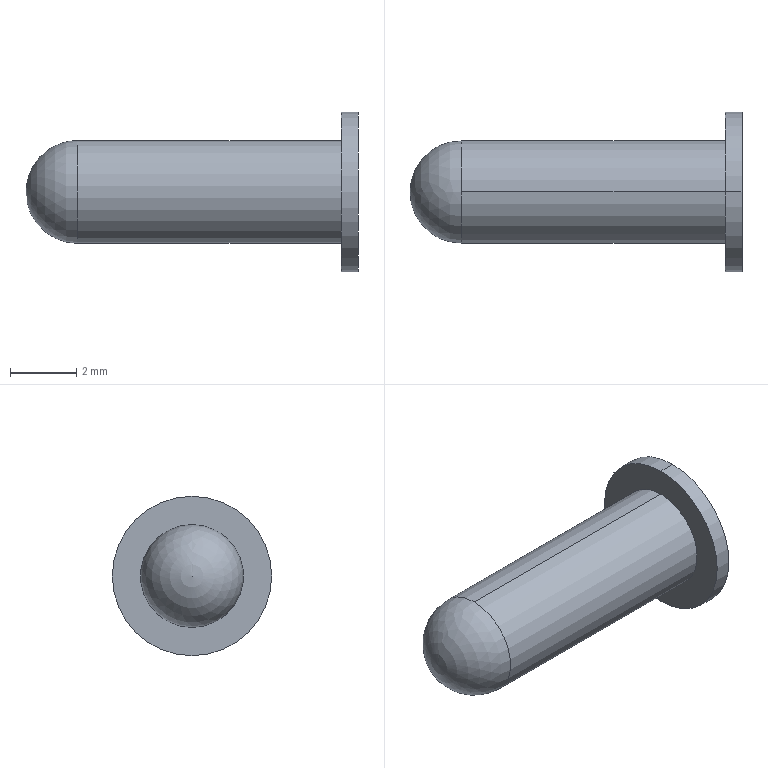Part | SolidWorks | features BaseBody 1 | 1 solid | 7 faces | box 10 x 4.8 x 4.8 mm | volume 76.851 mm3 | cylinder 4 | plane 2 | sphere 1 | commonest cylinder face diameters 3.1 x2 4.8 x2
STEP:
#1=CARTESIAN_POINT('',(-0.5,0.,1.55));
#2=VERTEX_POINT('',#1);
#3=CARTESIAN_POINT('',(-0.5,0.,-1.55));
#4=VERTEX_POINT('',#3);
#5=CARTESIAN_POINT('',(-0.5,0.,0.));
#6=DIRECTION('',(-1.,0.,0.));
#7=DIRECTION('',(0.,0.,1.));
#8=AXIS2_PLACEMENT_3D('',#5,#6,#7);
#9=CIRCLE('',#8,1.55);
#10=EDGE_CURVE('',#2,#4,#9,.T.);
#11=ORIENTED_EDGE('',*,*,#10,.T.);
#12=CARTESIAN_POINT('',(-8.45,0.,-1.55));
#13=VERTEX_POINT('',#12);
#14=CARTESIAN_POINT('',(0.,0.,-1.55));
#15=DIRECTION('',(-1.,0.,0.));
#16=VECTOR('',#15,1000.);
#17=LINE('',#14,#16);
#18=EDGE_CURVE('',#4,#13,#17,.T.);
#19=ORIENTED_EDGE('',*,*,#18,.T.);
#20=CARTESIAN_POINT('',(-8.45,0.,1.55));
#21=VERTEX_POINT('',#20);
#22=CARTESIAN_POINT('',(-8.45,0.,0.));
#23=DIRECTION('',(1.,0.,0.));
#24=DIRECTION('',(0.,0.,1.));
#25=AXIS2_PLACEMENT_3D('',#22,#23,#24);
#26=CIRCLE('',#25,1.55);
#27=EDGE_CURVE('',#13,#21,#26,.T.);
#28=ORIENTED_EDGE('',*,*,#27,.T.);
#29=CARTESIAN_POINT('',(0.,0.,1.55));
#30=DIRECTION('',(-1.,0.,0.));
#31=VECTOR('',#30,1000.);
#32=LINE('',#29,#31);
#33=EDGE_CURVE('',#2,#21,#32,.T.);
#34=ORIENTED_EDGE('',*,*,#33,.F.);
#35=EDGE_LOOP('',(#11,#19,#28,#34));
#36=FACE_OUTER_BOUND('',#35,.T.);
#37=CARTESIAN_POINT('',(0.,0.,0.));
#38=DIRECTION('',(-1.,0.,0.));
#39=DIRECTION('',(0.,0.,1.));
#40=AXIS2_PLACEMENT_3D('',#37,#38,#39);
#41=CYLINDRICAL_SURFACE('',#40,1.55);
#42=ADVANCED_FACE('',(#36),#41,.T.);
#43=CARTESIAN_POINT('',(0.,0.,2.4));
#44=VERTEX_POINT('',#43);
#45=CARTESIAN_POINT('',(0.,0.,-2.4));
#46=VERTEX_POINT('',#45);
#47=CARTESIAN_POINT('',(0.,0.,0.));
#48=DIRECTION('',(-1.,0.,0.));
#49=DIRECTION('',(0.,0.,1.));
#50=AXIS2_PLACEMENT_3D('',#47,#48,#49);
#51=CIRCLE('',#50,2.4);
#52=EDGE_CURVE('',#44,#46,#51,.T.);
#53=ORIENTED_EDGE('',*,*,#52,.T.);
#54=CARTESIAN_POINT('',(-0.5,0.,-2.4));
#55=VERTEX_POINT('',#54);
#56=CARTESIAN_POINT('',(0.,0.,-2.4));
#57=DIRECTION('',(-1.,0.,0.));
#58=VECTOR('',#57,1000.);
#59=LINE('',#56,#58);
#60=EDGE_CURVE('',#46,#55,#59,.T.);
#61=ORIENTED_EDGE('',*,*,#60,.T.);
#62=CARTESIAN_POINT('',(-0.5,0.,2.4));
#63=VERTEX_POINT('',#62);
#64=CARTESIAN_POINT('',(-0.5,0.,0.));
#65=DIRECTION('',(1.,0.,0.));
#66=DIRECTION('',(0.,0.,1.));
#67=AXIS2_PLACEMENT_3D('',#64,#65,#66);
#68=CIRCLE('',#67,2.4);
#69=EDGE_CURVE('',#55,#63,#68,.T.);
#70=ORIENTED_EDGE('',*,*,#69,.T.);
#71=CARTESIAN_POINT('',(0.,0.,2.4));
#72=DIRECTION('',(-1.,0.,0.));
#73=VECTOR('',#72,1000.);
#74=LINE('',#71,#73);
#75=EDGE_CURVE('',#44,#63,#74,.T.);
#76=ORIENTED_EDGE('',*,*,#75,.F.);
#77=EDGE_LOOP('',(#53,#61,#70,#76));
#78=FACE_OUTER_BOUND('',#77,.T.);
#79=CARTESIAN_POINT('',(0.,0.,0.));
#80=DIRECTION('',(-1.,0.,0.));
#81=DIRECTION('',(0.,0.,1.));
#82=AXIS2_PLACEMENT_3D('',#79,#80,#81);
#83=CYLINDRICAL_SURFACE('',#82,2.4);
#84=ADVANCED_FACE('',(#78),#83,.T.);
#85=ORIENTED_EDGE('',*,*,#18,.F.);
#86=CARTESIAN_POINT('',(-0.5,0.,0.));
#87=DIRECTION('',(-1.,0.,0.));
#88=DIRECTION('',(0.,0.,1.));
#89=AXIS2_PLACEMENT_3D('',#86,#87,#88);
#90=CIRCLE('',#89,1.55);
#91=EDGE_CURVE('',#4,#2,#90,.T.);
#92=ORIENTED_EDGE('',*,*,#91,.T.);
#93=ORIENTED_EDGE('',*,*,#33,.T.);
#94=CARTESIAN_POINT('',(-8.45,0.,0.));
#95=DIRECTION('',(1.,0.,0.));
#96=DIRECTION('',(0.,0.,1.));
#97=AXIS2_PLACEMENT_3D('',#94,#95,#96);
#98=CIRCLE('',#97,1.55);
#99=EDGE_CURVE('',#21,#13,#98,.T.);
#100=ORIENTED_EDGE('',*,*,#99,.T.);
#101=EDGE_LOOP('',(#85,#92,#93,#100));
#102=FACE_OUTER_BOUND('',#101,.T.);
#103=CARTESIAN_POINT('',(0.,0.,0.));
#104=DIRECTION('',(-1.,0.,0.));
#105=DIRECTION('',(0.,0.,1.));
#106=AXIS2_PLACEMENT_3D('',#103,#104,#105);
#107=CYLINDRICAL_SURFACE('',#106,1.55);
#108=ADVANCED_FACE('',(#102),#107,.T.);
#109=ORIENTED_EDGE('',*,*,#99,.F.);
#110=ORIENTED_EDGE('',*,*,#27,.F.);
#111=EDGE_LOOP('',(#109,#110));
#112=FACE_OUTER_BOUND('',#111,.T.);
#113=CARTESIAN_POINT('',(-8.45,0.,0.));
#114=DIRECTION('',(1.,0.,0.));
#115=DIRECTION('',(0.,0.,1.));
#116=AXIS2_PLACEMENT_3D('',#113,#114,#115);
#117=SPHERICAL_SURFACE('',#116,1.55);
#118=ADVANCED_FACE('',(#112),#117,.T.);
#119=CARTESIAN_POINT('',(-0.5,0.,0.));
#120=DIRECTION('',(1.,0.,0.));
#121=DIRECTION('',(0.,0.,1.));
#122=AXIS2_PLACEMENT_3D('',#119,#120,#121);
#123=CIRCLE('',#122,2.4);
#124=EDGE_CURVE('',#63,#55,#123,.T.);
#125=ORIENTED_EDGE('',*,*,#124,.F.);
#126=ORIENTED_EDGE('',*,*,#69,.F.);
#127=EDGE_LOOP('',(#125,#126));
#128=FACE_OUTER_BOUND('',#127,.T.);
#129=ORIENTED_EDGE('',*,*,#10,.F.);
#130=ORIENTED_EDGE('',*,*,#91,.F.);
#131=EDGE_LOOP('',(#129,#130));
#132=FACE_BOUND('',#131,.T.);
#133=CARTESIAN_POINT('',(-0.5,1.55,0.));
#134=DIRECTION('',(1.,0.,0.));
#135=DIRECTION('',(0.,0.,-1.));
#136=AXIS2_PLACEMENT_3D('',#133,#134,#135);
#137=PLANE('',#136);
#138=ADVANCED_FACE('',(#128,#132),#137,.F.);
#139=ORIENTED_EDGE('',*,*,#60,.F.);
#140=CARTESIAN_POINT('',(0.,0.,0.));
#141=DIRECTION('',(-1.,0.,0.));
#142=DIRECTION('',(0.,0.,1.));
#143=AXIS2_PLACEMENT_3D('',#140,#141,#142);
#144=CIRCLE('',#143,2.4);
#145=EDGE_CURVE('',#46,#44,#144,.T.);
#146=ORIENTED_EDGE('',*,*,#145,.T.);
#147=ORIENTED_EDGE('',*,*,#75,.T.);
#148=ORIENTED_EDGE('',*,*,#124,.T.);
#149=EDGE_LOOP('',(#139,#146,#147,#148));
#150=FACE_OUTER_BOUND('',#149,.T.);
#151=CARTESIAN_POINT('',(0.,0.,0.));
#152=DIRECTION('',(-1.,0.,0.));
#153=DIRECTION('',(0.,0.,1.));
#154=AXIS2_PLACEMENT_3D('',#151,#152,#153);
#155=CYLINDRICAL_SURFACE('',#154,2.4);
#156=ADVANCED_FACE('',(#150),#155,.T.);
#157=ORIENTED_EDGE('',*,*,#52,.F.);
#158=ORIENTED_EDGE('',*,*,#145,.F.);
#159=EDGE_LOOP('',(#157,#158));
#160=FACE_OUTER_BOUND('',#159,.T.);
#161=CARTESIAN_POINT('',(0.,2.4,0.));
#162=DIRECTION('',(-1.,0.,0.));
#163=DIRECTION('',(0.,0.,1.));
#164=AXIS2_PLACEMENT_3D('',#161,#162,#163);
#165=PLANE('',#164);
#166=ADVANCED_FACE('',(#160),#165,.F.);
#167=CLOSED_SHELL('',(#42,#84,#108,#118,#138,#156,#166));
#168=MANIFOLD_SOLID_BREP('',#167);
#169=CARTESIAN_POINT('',(0.,0.,0.));
#170=DIRECTION('',(0.,0.,1.));
#171=DIRECTION('',(1.,0.,0.));
#172=AXIS2_PLACEMENT_3D('',#169,#170,#171);
#173=(LENGTH_UNIT()NAMED_UNIT(*)SI_UNIT(.MILLI.,.METRE.));
#174=UNCERTAINTY_MEASURE_WITH_UNIT(LENGTH_MEASURE(0.00001),#173,'','');
#175=(NAMED_UNIT(*)PLANE_ANGLE_UNIT()SI_UNIT($,.RADIAN.));
#176=(NAMED_UNIT(*)SI_UNIT($,.STERADIAN.)SOLID_ANGLE_UNIT());
#177=(GEOMETRIC_REPRESENTATION_CONTEXT(3)GLOBAL_UNCERTAINTY_ASSIGNED_CONTEXT((#174))GLOBAL_UNIT_ASSIGNED_CONTEXT((#173,#175,#176))REPRESENTATION_CONTEXT('',''));
#178=ADVANCED_BREP_SHAPE_REPRESENTATION('',(#168,#172),#177);